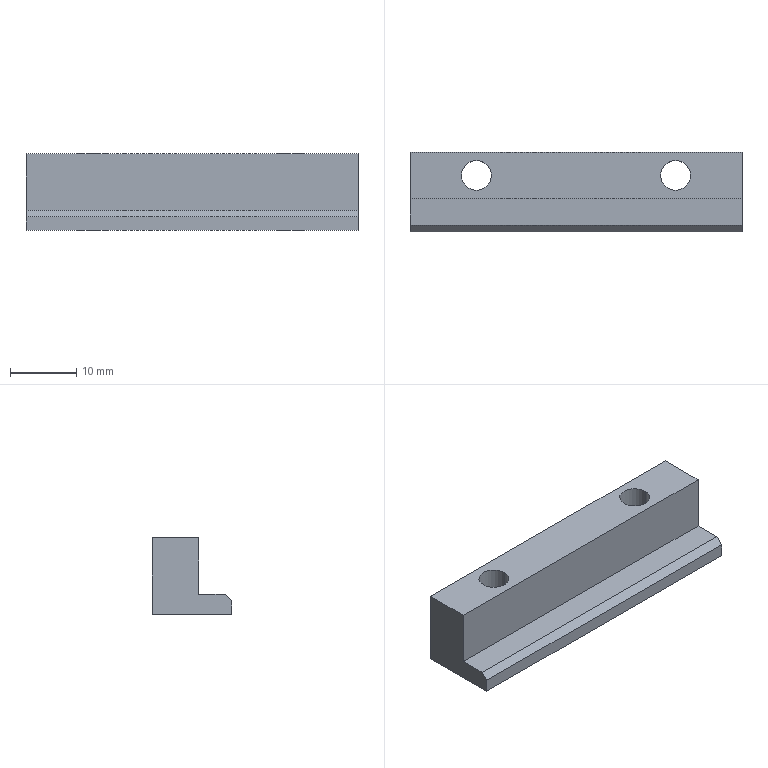Part | SolidWorks | features ICE 2, Chamfer 1, Extrusion 1, MoveFace 1 | 1 solid | 13 faces | box 50 x 12 x 11.5 mm | volume 4384 mm3 | plane 9 | cylinder 4 | commonest cylinder face diameters 4.5 x4
STEP:
#1=CARTESIAN_POINT('',(7.75,8.5,0.));
#2=VERTEX_POINT('',#1);
#3=CARTESIAN_POINT('',(12.25,8.5,0.));
#4=VERTEX_POINT('',#3);
#5=CARTESIAN_POINT('',(10.,8.5,0.));
#6=DIRECTION('',(0.,0.,1.));
#7=DIRECTION('',(1.,0.,0.));
#8=AXIS2_PLACEMENT_3D('',#5,#6,#7);
#9=CIRCLE('',#8,2.25);
#10=EDGE_CURVE('',#2,#4,#9,.T.);
#11=ORIENTED_EDGE('',*,*,#10,.F.);
#12=CARTESIAN_POINT('',(7.75,8.5,11.5));
#13=VERTEX_POINT('',#12);
#14=CARTESIAN_POINT('',(7.75,8.5,0.));
#15=DIRECTION('',(0.,0.,1.));
#16=VECTOR('',#15,1000.);
#17=LINE('',#14,#16);
#18=EDGE_CURVE('',#2,#13,#17,.T.);
#19=ORIENTED_EDGE('',*,*,#18,.T.);
#20=CARTESIAN_POINT('',(12.25,8.5,11.5));
#21=VERTEX_POINT('',#20);
#22=CARTESIAN_POINT('',(10.,8.5,11.5));
#23=DIRECTION('',(0.,0.,1.));
#24=DIRECTION('',(1.,0.,0.));
#25=AXIS2_PLACEMENT_3D('',#22,#23,#24);
#26=CIRCLE('',#25,2.25);
#27=EDGE_CURVE('',#13,#21,#26,.T.);
#28=ORIENTED_EDGE('',*,*,#27,.T.);
#29=CARTESIAN_POINT('',(12.25,8.5,0.));
#30=DIRECTION('',(0.,0.,1.));
#31=VECTOR('',#30,1000.);
#32=LINE('',#29,#31);
#33=EDGE_CURVE('',#4,#21,#32,.T.);
#34=ORIENTED_EDGE('',*,*,#33,.F.);
#35=EDGE_LOOP('',(#11,#19,#28,#34));
#36=FACE_OUTER_BOUND('',#35,.T.);
#37=CARTESIAN_POINT('',(10.,8.5,0.));
#38=DIRECTION('',(0.,0.,1.));
#39=DIRECTION('',(1.,0.,0.));
#40=AXIS2_PLACEMENT_3D('',#37,#38,#39);
#41=CYLINDRICAL_SURFACE('',#40,2.25);
#42=ADVANCED_FACE('',(#36),#41,.F.);
#43=CARTESIAN_POINT('',(37.75,8.5,0.));
#44=VERTEX_POINT('',#43);
#45=CARTESIAN_POINT('',(42.25,8.5,0.));
#46=VERTEX_POINT('',#45);
#47=CARTESIAN_POINT('',(40.,8.5,0.));
#48=DIRECTION('',(0.,0.,1.));
#49=DIRECTION('',(1.,0.,0.));
#50=AXIS2_PLACEMENT_3D('',#47,#48,#49);
#51=CIRCLE('',#50,2.25);
#52=EDGE_CURVE('',#44,#46,#51,.T.);
#53=ORIENTED_EDGE('',*,*,#52,.F.);
#54=CARTESIAN_POINT('',(37.75,8.5,11.5));
#55=VERTEX_POINT('',#54);
#56=CARTESIAN_POINT('',(37.75,8.5,0.));
#57=DIRECTION('',(0.,0.,1.));
#58=VECTOR('',#57,1000.);
#59=LINE('',#56,#58);
#60=EDGE_CURVE('',#44,#55,#59,.T.);
#61=ORIENTED_EDGE('',*,*,#60,.T.);
#62=CARTESIAN_POINT('',(42.25,8.5,11.5));
#63=VERTEX_POINT('',#62);
#64=CARTESIAN_POINT('',(40.,8.5,11.5));
#65=DIRECTION('',(0.,0.,1.));
#66=DIRECTION('',(1.,0.,0.));
#67=AXIS2_PLACEMENT_3D('',#64,#65,#66);
#68=CIRCLE('',#67,2.25);
#69=EDGE_CURVE('',#55,#63,#68,.T.);
#70=ORIENTED_EDGE('',*,*,#69,.T.);
#71=CARTESIAN_POINT('',(42.25,8.5,0.));
#72=DIRECTION('',(0.,0.,1.));
#73=VECTOR('',#72,1000.);
#74=LINE('',#71,#73);
#75=EDGE_CURVE('',#46,#63,#74,.T.);
#76=ORIENTED_EDGE('',*,*,#75,.F.);
#77=EDGE_LOOP('',(#53,#61,#70,#76));
#78=FACE_OUTER_BOUND('',#77,.T.);
#79=CARTESIAN_POINT('',(40.,8.5,0.));
#80=DIRECTION('',(0.,0.,1.));
#81=DIRECTION('',(1.,0.,0.));
#82=AXIS2_PLACEMENT_3D('',#79,#80,#81);
#83=CYLINDRICAL_SURFACE('',#82,2.25);
#84=ADVANCED_FACE('',(#78),#83,.F.);
#85=CARTESIAN_POINT('',(0.,0.,2.));
#86=VERTEX_POINT('',#85);
#87=CARTESIAN_POINT('',(0.,0.,0.));
#88=VERTEX_POINT('',#87);
#89=CARTESIAN_POINT('',(0.,0.,5.));
#90=DIRECTION('',(0.,0.,-1.));
#91=VECTOR('',#90,1000.);
#92=LINE('',#89,#91);
#93=EDGE_CURVE('',#86,#88,#92,.T.);
#94=ORIENTED_EDGE('',*,*,#93,.F.);
#95=CARTESIAN_POINT('',(0.,1.,3.));
#96=VERTEX_POINT('',#95);
#97=CARTESIAN_POINT('',(0.,1.,3.));
#98=DIRECTION('',(0.,0.7071,0.7071));
#99=VECTOR('',#98,1000.);
#100=LINE('',#97,#99);
#101=EDGE_CURVE('',#86,#96,#100,.T.);
#102=ORIENTED_EDGE('',*,*,#101,.T.);
#103=CARTESIAN_POINT('',(0.,5.,3.));
#104=VERTEX_POINT('',#103);
#105=CARTESIAN_POINT('',(0.,0.,3.));
#106=DIRECTION('',(0.,1.,0.));
#107=VECTOR('',#106,1000.);
#108=LINE('',#105,#107);
#109=EDGE_CURVE('',#96,#104,#108,.T.);
#110=ORIENTED_EDGE('',*,*,#109,.T.);
#111=CARTESIAN_POINT('',(0.,5.,11.5));
#112=VERTEX_POINT('',#111);
#113=CARTESIAN_POINT('',(0.,5.,5.));
#114=DIRECTION('',(0.,0.,1.));
#115=VECTOR('',#114,1000.);
#116=LINE('',#113,#115);
#117=EDGE_CURVE('',#104,#112,#116,.T.);
#118=ORIENTED_EDGE('',*,*,#117,.T.);
#119=CARTESIAN_POINT('',(0.,12.,11.5));
#120=VERTEX_POINT('',#119);
#121=CARTESIAN_POINT('',(0.,0.,11.5));
#122=DIRECTION('',(0.,-1.,0.));
#123=VECTOR('',#122,1000.);
#124=LINE('',#121,#123);
#125=EDGE_CURVE('',#120,#112,#124,.T.);
#126=ORIENTED_EDGE('',*,*,#125,.F.);
#127=CARTESIAN_POINT('',(0.,12.,0.));
#128=VERTEX_POINT('',#127);
#129=CARTESIAN_POINT('',(0.,12.,5.));
#130=DIRECTION('',(0.,0.,-1.));
#131=VECTOR('',#130,1000.);
#132=LINE('',#129,#131);
#133=EDGE_CURVE('',#120,#128,#132,.T.);
#134=ORIENTED_EDGE('',*,*,#133,.T.);
#135=CARTESIAN_POINT('',(0.,0.,0.));
#136=DIRECTION('',(0.,-1.,0.));
#137=VECTOR('',#136,1000.);
#138=LINE('',#135,#137);
#139=EDGE_CURVE('',#128,#88,#138,.T.);
#140=ORIENTED_EDGE('',*,*,#139,.T.);
#141=EDGE_LOOP('',(#94,#102,#110,#118,#126,#134,#140));
#142=FACE_OUTER_BOUND('',#141,.T.);
#143=CARTESIAN_POINT('',(0.,0.,5.));
#144=DIRECTION('',(1.,0.,0.));
#145=DIRECTION('',(0.,0.,-1.));
#146=AXIS2_PLACEMENT_3D('',#143,#144,#145);
#147=PLANE('',#146);
#148=ADVANCED_FACE('',(#142),#147,.F.);
#149=CARTESIAN_POINT('',(50.,0.,2.));
#150=VERTEX_POINT('',#149);
#151=CARTESIAN_POINT('',(50.,0.,0.));
#152=VERTEX_POINT('',#151);
#153=CARTESIAN_POINT('',(50.,0.,5.));
#154=DIRECTION('',(0.,0.,-1.));
#155=VECTOR('',#154,1000.);
#156=LINE('',#153,#155);
#157=EDGE_CURVE('',#150,#152,#156,.T.);
#158=ORIENTED_EDGE('',*,*,#157,.F.);
#159=CARTESIAN_POINT('',(0.,0.,2.));
#160=DIRECTION('',(-1.,0.,0.));
#161=VECTOR('',#160,1000.);
#162=LINE('',#159,#161);
#163=EDGE_CURVE('',#150,#86,#162,.T.);
#164=ORIENTED_EDGE('',*,*,#163,.T.);
#165=ORIENTED_EDGE('',*,*,#93,.T.);
#166=CARTESIAN_POINT('',(0.,0.,0.));
#167=DIRECTION('',(1.,0.,0.));
#168=VECTOR('',#167,1000.);
#169=LINE('',#166,#168);
#170=EDGE_CURVE('',#88,#152,#169,.T.);
#171=ORIENTED_EDGE('',*,*,#170,.T.);
#172=EDGE_LOOP('',(#158,#164,#165,#171));
#173=FACE_OUTER_BOUND('',#172,.T.);
#174=CARTESIAN_POINT('',(0.,0.,5.));
#175=DIRECTION('',(0.,1.,0.));
#176=DIRECTION('',(0.,0.,1.));
#177=AXIS2_PLACEMENT_3D('',#174,#175,#176);
#178=PLANE('',#177);
#179=ADVANCED_FACE('',(#173),#178,.F.);
#180=CARTESIAN_POINT('',(50.,1.,3.));
#181=VERTEX_POINT('',#180);
#182=CARTESIAN_POINT('',(50.,5.,3.));
#183=VERTEX_POINT('',#182);
#184=CARTESIAN_POINT('',(50.,0.,3.));
#185=DIRECTION('',(0.,1.,0.));
#186=VECTOR('',#185,1000.);
#187=LINE('',#184,#186);
#188=EDGE_CURVE('',#181,#183,#187,.T.);
#189=ORIENTED_EDGE('',*,*,#188,.F.);
#190=CARTESIAN_POINT('',(50.,1.,3.));
#191=DIRECTION('',(0.,-0.7071,-0.7071));
#192=VECTOR('',#191,1000.);
#193=LINE('',#190,#192);
#194=EDGE_CURVE('',#181,#150,#193,.T.);
#195=ORIENTED_EDGE('',*,*,#194,.T.);
#196=ORIENTED_EDGE('',*,*,#157,.T.);
#197=CARTESIAN_POINT('',(50.,12.,0.));
#198=VERTEX_POINT('',#197);
#199=CARTESIAN_POINT('',(50.,0.,0.));
#200=DIRECTION('',(0.,1.,0.));
#201=VECTOR('',#200,1000.);
#202=LINE('',#199,#201);
#203=EDGE_CURVE('',#152,#198,#202,.T.);
#204=ORIENTED_EDGE('',*,*,#203,.T.);
#205=CARTESIAN_POINT('',(50.,12.,11.5));
#206=VERTEX_POINT('',#205);
#207=CARTESIAN_POINT('',(50.,12.,5.));
#208=DIRECTION('',(0.,0.,-1.));
#209=VECTOR('',#208,1000.);
#210=LINE('',#207,#209);
#211=EDGE_CURVE('',#206,#198,#210,.T.);
#212=ORIENTED_EDGE('',*,*,#211,.F.);
#213=CARTESIAN_POINT('',(50.,5.,11.5));
#214=VERTEX_POINT('',#213);
#215=CARTESIAN_POINT('',(50.,0.,11.5));
#216=DIRECTION('',(0.,1.,0.));
#217=VECTOR('',#216,1000.);
#218=LINE('',#215,#217);
#219=EDGE_CURVE('',#214,#206,#218,.T.);
#220=ORIENTED_EDGE('',*,*,#219,.F.);
#221=CARTESIAN_POINT('',(50.,5.,5.));
#222=DIRECTION('',(0.,0.,1.));
#223=VECTOR('',#222,1000.);
#224=LINE('',#221,#223);
#225=EDGE_CURVE('',#183,#214,#224,.T.);
#226=ORIENTED_EDGE('',*,*,#225,.F.);
#227=EDGE_LOOP('',(#189,#195,#196,#204,#212,#220,#226));
#228=FACE_OUTER_BOUND('',#227,.T.);
#229=CARTESIAN_POINT('',(50.,0.,5.));
#230=DIRECTION('',(-1.,0.,0.));
#231=DIRECTION('',(0.,0.,1.));
#232=AXIS2_PLACEMENT_3D('',#229,#230,#231);
#233=PLANE('',#232);
#234=ADVANCED_FACE('',(#228),#233,.F.);
#235=CARTESIAN_POINT('',(0.,12.,0.));
#236=DIRECTION('',(-1.,0.,0.));
#237=VECTOR('',#236,1000.);
#238=LINE('',#235,#237);
#239=EDGE_CURVE('',#198,#128,#238,.T.);
#240=ORIENTED_EDGE('',*,*,#239,.T.);
#241=ORIENTED_EDGE('',*,*,#133,.F.);
#242=CARTESIAN_POINT('',(0.,12.,11.5));
#243=DIRECTION('',(-1.,0.,0.));
#244=VECTOR('',#243,1000.);
#245=LINE('',#242,#244);
#246=EDGE_CURVE('',#206,#120,#245,.T.);
#247=ORIENTED_EDGE('',*,*,#246,.F.);
#248=ORIENTED_EDGE('',*,*,#211,.T.);
#249=EDGE_LOOP('',(#240,#241,#247,#248));
#250=FACE_OUTER_BOUND('',#249,.T.);
#251=CARTESIAN_POINT('',(0.,12.,5.));
#252=DIRECTION('',(0.,-1.,0.));
#253=DIRECTION('',(0.,0.,-1.));
#254=AXIS2_PLACEMENT_3D('',#251,#252,#253);
#255=PLANE('',#254);
#256=ADVANCED_FACE('',(#250),#255,.F.);
#257=CARTESIAN_POINT('',(10.,8.5,11.5));
#258=DIRECTION('',(0.,0.,1.));
#259=DIRECTION('',(1.,0.,0.));
#260=AXIS2_PLACEMENT_3D('',#257,#258,#259);
#261=CIRCLE('',#260,2.25);
#262=EDGE_CURVE('',#21,#13,#261,.T.);
#263=ORIENTED_EDGE('',*,*,#262,.F.);
#264=ORIENTED_EDGE('',*,*,#27,.F.);
#265=EDGE_LOOP('',(#263,#264));
#266=FACE_BOUND('',#265,.T.);
#267=CARTESIAN_POINT('',(40.,8.5,11.5));
#268=DIRECTION('',(0.,0.,1.));
#269=DIRECTION('',(1.,0.,0.));
#270=AXIS2_PLACEMENT_3D('',#267,#268,#269);
#271=CIRCLE('',#270,2.25);
#272=EDGE_CURVE('',#63,#55,#271,.T.);
#273=ORIENTED_EDGE('',*,*,#272,.F.);
#274=ORIENTED_EDGE('',*,*,#69,.F.);
#275=EDGE_LOOP('',(#273,#274));
#276=FACE_BOUND('',#275,.T.);
#277=ORIENTED_EDGE('',*,*,#125,.T.);
#278=CARTESIAN_POINT('',(0.,5.,11.5));
#279=DIRECTION('',(1.,0.,0.));
#280=VECTOR('',#279,1000.);
#281=LINE('',#278,#280);
#282=EDGE_CURVE('',#112,#214,#281,.T.);
#283=ORIENTED_EDGE('',*,*,#282,.T.);
#284=ORIENTED_EDGE('',*,*,#219,.T.);
#285=ORIENTED_EDGE('',*,*,#246,.T.);
#286=EDGE_LOOP('',(#277,#283,#284,#285));
#287=FACE_OUTER_BOUND('',#286,.T.);
#288=CARTESIAN_POINT('',(0.,0.,11.5));
#289=DIRECTION('',(0.,0.,-1.));
#290=DIRECTION('',(-1.,0.,0.));
#291=AXIS2_PLACEMENT_3D('',#288,#289,#290);
#292=PLANE('',#291);
#293=ADVANCED_FACE('',(#266,#276,#287),#292,.F.);
#294=CARTESIAN_POINT('',(10.,8.5,0.));
#295=DIRECTION('',(0.,0.,1.));
#296=DIRECTION('',(1.,0.,0.));
#297=AXIS2_PLACEMENT_3D('',#294,#295,#296);
#298=CIRCLE('',#297,2.25);
#299=EDGE_CURVE('',#4,#2,#298,.T.);
#300=ORIENTED_EDGE('',*,*,#299,.T.);
#301=ORIENTED_EDGE('',*,*,#10,.T.);
#302=EDGE_LOOP('',(#300,#301));
#303=FACE_BOUND('',#302,.T.);
#304=CARTESIAN_POINT('',(40.,8.5,0.));
#305=DIRECTION('',(0.,0.,1.));
#306=DIRECTION('',(1.,0.,0.));
#307=AXIS2_PLACEMENT_3D('',#304,#305,#306);
#308=CIRCLE('',#307,2.25);
#309=EDGE_CURVE('',#46,#44,#308,.T.);
#310=ORIENTED_EDGE('',*,*,#309,.T.);
#311=ORIENTED_EDGE('',*,*,#52,.T.);
#312=EDGE_LOOP('',(#310,#311));
#313=FACE_BOUND('',#312,.T.);
#314=ORIENTED_EDGE('',*,*,#139,.F.);
#315=ORIENTED_EDGE('',*,*,#239,.F.);
#316=ORIENTED_EDGE('',*,*,#203,.F.);
#317=ORIENTED_EDGE('',*,*,#170,.F.);
#318=EDGE_LOOP('',(#314,#315,#316,#317));
#319=FACE_OUTER_BOUND('',#318,.T.);
#320=CARTESIAN_POINT('',(0.,0.,0.));
#321=DIRECTION('',(0.,0.,-1.));
#322=DIRECTION('',(-1.,0.,0.));
#323=AXIS2_PLACEMENT_3D('',#320,#321,#322);
#324=PLANE('',#323);
#325=ADVANCED_FACE('',(#303,#313,#319),#324,.T.);
#326=ORIENTED_EDGE('',*,*,#60,.F.);
#327=ORIENTED_EDGE('',*,*,#309,.F.);
#328=ORIENTED_EDGE('',*,*,#75,.T.);
#329=ORIENTED_EDGE('',*,*,#272,.T.);
#330=EDGE_LOOP('',(#326,#327,#328,#329));
#331=FACE_OUTER_BOUND('',#330,.T.);
#332=CARTESIAN_POINT('',(40.,8.5,0.));
#333=DIRECTION('',(0.,0.,1.));
#334=DIRECTION('',(1.,0.,0.));
#335=AXIS2_PLACEMENT_3D('',#332,#333,#334);
#336=CYLINDRICAL_SURFACE('',#335,2.25);
#337=ADVANCED_FACE('',(#331),#336,.F.);
#338=ORIENTED_EDGE('',*,*,#18,.F.);
#339=ORIENTED_EDGE('',*,*,#299,.F.);
#340=ORIENTED_EDGE('',*,*,#33,.T.);
#341=ORIENTED_EDGE('',*,*,#262,.T.);
#342=EDGE_LOOP('',(#338,#339,#340,#341));
#343=FACE_OUTER_BOUND('',#342,.T.);
#344=CARTESIAN_POINT('',(10.,8.5,0.));
#345=DIRECTION('',(0.,0.,1.));
#346=DIRECTION('',(1.,0.,0.));
#347=AXIS2_PLACEMENT_3D('',#344,#345,#346);
#348=CYLINDRICAL_SURFACE('',#347,2.25);
#349=ADVANCED_FACE('',(#343),#348,.F.);
#350=ORIENTED_EDGE('',*,*,#225,.T.);
#351=ORIENTED_EDGE('',*,*,#282,.F.);
#352=ORIENTED_EDGE('',*,*,#117,.F.);
#353=CARTESIAN_POINT('',(0.,5.,3.));
#354=DIRECTION('',(1.,0.,0.));
#355=VECTOR('',#354,1000.);
#356=LINE('',#353,#355);
#357=EDGE_CURVE('',#104,#183,#356,.T.);
#358=ORIENTED_EDGE('',*,*,#357,.T.);
#359=EDGE_LOOP('',(#350,#351,#352,#358));
#360=FACE_OUTER_BOUND('',#359,.T.);
#361=CARTESIAN_POINT('',(0.,5.,5.));
#362=DIRECTION('',(0.,1.,0.));
#363=DIRECTION('',(0.,0.,1.));
#364=AXIS2_PLACEMENT_3D('',#361,#362,#363);
#365=PLANE('',#364);
#366=ADVANCED_FACE('',(#360),#365,.F.);
#367=ORIENTED_EDGE('',*,*,#109,.F.);
#368=CARTESIAN_POINT('',(0.,1.,3.));
#369=DIRECTION('',(1.,0.,0.));
#370=VECTOR('',#369,1000.);
#371=LINE('',#368,#370);
#372=EDGE_CURVE('',#96,#181,#371,.T.);
#373=ORIENTED_EDGE('',*,*,#372,.T.);
#374=ORIENTED_EDGE('',*,*,#188,.T.);
#375=ORIENTED_EDGE('',*,*,#357,.F.);
#376=EDGE_LOOP('',(#367,#373,#374,#375));
#377=FACE_OUTER_BOUND('',#376,.T.);
#378=CARTESIAN_POINT('',(0.,0.,3.));
#379=DIRECTION('',(0.,0.,-1.));
#380=DIRECTION('',(-1.,0.,0.));
#381=AXIS2_PLACEMENT_3D('',#378,#379,#380);
#382=PLANE('',#381);
#383=ADVANCED_FACE('',(#377),#382,.F.);
#384=ORIENTED_EDGE('',*,*,#101,.F.);
#385=ORIENTED_EDGE('',*,*,#163,.F.);
#386=ORIENTED_EDGE('',*,*,#194,.F.);
#387=ORIENTED_EDGE('',*,*,#372,.F.);
#388=EDGE_LOOP('',(#384,#385,#386,#387));
#389=FACE_OUTER_BOUND('',#388,.T.);
#390=CARTESIAN_POINT('',(0.,1.,3.));
#391=DIRECTION('',(0.,0.7071,-0.7071));
#392=DIRECTION('',(1.,0.,0.));
#393=AXIS2_PLACEMENT_3D('',#390,#391,#392);
#394=PLANE('',#393);
#395=ADVANCED_FACE('',(#389),#394,.F.);
#396=CLOSED_SHELL('',(#42,#84,#148,#179,#234,#256,#293,#325,#337,#349,#366,#383,#395));
#397=MANIFOLD_SOLID_BREP('',#396);
#398=CARTESIAN_POINT('',(0.,0.,0.));
#399=DIRECTION('',(0.,0.,1.));
#400=DIRECTION('',(1.,0.,0.));
#401=AXIS2_PLACEMENT_3D('',#398,#399,#400);
#402=(LENGTH_UNIT()NAMED_UNIT(*)SI_UNIT(.MILLI.,.METRE.));
#403=UNCERTAINTY_MEASURE_WITH_UNIT(LENGTH_MEASURE(0.00001),#402,'','');
#404=(NAMED_UNIT(*)PLANE_ANGLE_UNIT()SI_UNIT($,.RADIAN.));
#405=(NAMED_UNIT(*)SI_UNIT($,.STERADIAN.)SOLID_ANGLE_UNIT());
#406=(GEOMETRIC_REPRESENTATION_CONTEXT(3)GLOBAL_UNCERTAINTY_ASSIGNED_CONTEXT((#403))GLOBAL_UNIT_ASSIGNED_CONTEXT((#402,#404,#405))REPRESENTATION_CONTEXT('',''));
#407=ADVANCED_BREP_SHAPE_REPRESENTATION('',(#397,#401),#406);